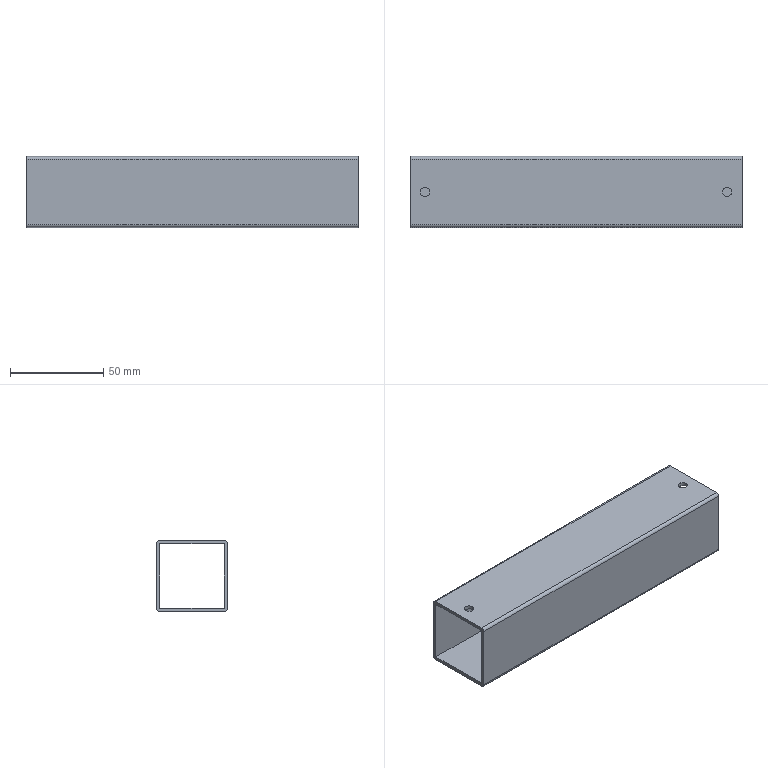Part | NX | features BREP 1 | 1 solid | 18 faces | box 177.8 x 38.1 x 38.1 mm | volume 47962 mm3 | plane 10 | cylinder 8 | commonest cylinder face diameters 3.175 x4 4.826 x2 5.029 x2
STEP:
#1=CARTESIAN_POINT('',(-88.9,19.05,-17.462));
#2=VERTEX_POINT('',#1);
#3=CARTESIAN_POINT('',(-88.9,19.05,17.462));
#4=VERTEX_POINT('',#3);
#5=CARTESIAN_POINT('',(-88.9,19.05,-17.462));
#6=DIRECTION('',(0.,0.,1.));
#7=VECTOR('',#6,1000.);
#8=LINE('',#5,#7);
#9=EDGE_CURVE('',#2,#4,#8,.T.);
#10=ORIENTED_EDGE('',*,*,#9,.F.);
#11=CARTESIAN_POINT('',(-88.9,17.462,-19.05));
#12=VERTEX_POINT('',#11);
#13=CARTESIAN_POINT('',(-88.9,17.462,-17.462));
#14=DIRECTION('',(-1.,0.,0.));
#15=DIRECTION('',(0.,1.,0.));
#16=AXIS2_PLACEMENT_3D('',#13,#14,#15);
#17=CIRCLE('',#16,1.587);
#18=EDGE_CURVE('',#2,#12,#17,.T.);
#19=ORIENTED_EDGE('',*,*,#18,.T.);
#20=CARTESIAN_POINT('',(-88.9,-17.462,-19.05));
#21=VERTEX_POINT('',#20);
#22=CARTESIAN_POINT('',(-88.9,-17.462,-19.05));
#23=DIRECTION('',(0.,1.,0.));
#24=VECTOR('',#23,1000.);
#25=LINE('',#22,#24);
#26=EDGE_CURVE('',#21,#12,#25,.T.);
#27=ORIENTED_EDGE('',*,*,#26,.F.);
#28=CARTESIAN_POINT('',(-88.9,-19.05,-17.462));
#29=VERTEX_POINT('',#28);
#30=CARTESIAN_POINT('',(-88.9,-17.462,-17.462));
#31=DIRECTION('',(-1.,0.,0.));
#32=DIRECTION('',(0.,0.,-1.));
#33=AXIS2_PLACEMENT_3D('',#30,#31,#32);
#34=CIRCLE('',#33,1.587);
#35=EDGE_CURVE('',#21,#29,#34,.T.);
#36=ORIENTED_EDGE('',*,*,#35,.T.);
#37=CARTESIAN_POINT('',(-88.9,-19.05,17.462));
#38=VERTEX_POINT('',#37);
#39=CARTESIAN_POINT('',(-88.9,-19.05,17.462));
#40=DIRECTION('',(0.,0.,-1.));
#41=VECTOR('',#40,1000.);
#42=LINE('',#39,#41);
#43=EDGE_CURVE('',#38,#29,#42,.T.);
#44=ORIENTED_EDGE('',*,*,#43,.F.);
#45=CARTESIAN_POINT('',(-88.9,-17.462,19.05));
#46=VERTEX_POINT('',#45);
#47=CARTESIAN_POINT('',(-88.9,-17.462,17.462));
#48=DIRECTION('',(-1.,0.,0.));
#49=DIRECTION('',(0.,-1.,0.));
#50=AXIS2_PLACEMENT_3D('',#47,#48,#49);
#51=CIRCLE('',#50,1.587);
#52=EDGE_CURVE('',#38,#46,#51,.T.);
#53=ORIENTED_EDGE('',*,*,#52,.T.);
#54=CARTESIAN_POINT('',(-88.9,17.462,19.05));
#55=VERTEX_POINT('',#54);
#56=CARTESIAN_POINT('',(-88.9,17.462,19.05));
#57=DIRECTION('',(0.,-1.,0.));
#58=VECTOR('',#57,1000.);
#59=LINE('',#56,#58);
#60=EDGE_CURVE('',#55,#46,#59,.T.);
#61=ORIENTED_EDGE('',*,*,#60,.F.);
#62=CARTESIAN_POINT('',(-88.9,17.462,17.462));
#63=DIRECTION('',(-1.,0.,0.));
#64=DIRECTION('',(0.,0.,1.));
#65=AXIS2_PLACEMENT_3D('',#62,#63,#64);
#66=CIRCLE('',#65,1.587);
#67=EDGE_CURVE('',#55,#4,#66,.T.);
#68=ORIENTED_EDGE('',*,*,#67,.T.);
#69=EDGE_LOOP('',(#10,#19,#27,#36,#44,#53,#61,#68));
#70=FACE_BOUND('',#69,.T.);
#71=CARTESIAN_POINT('',(-88.9,17.17,17.17));
#72=VERTEX_POINT('',#71);
#73=CARTESIAN_POINT('',(-88.9,17.17,-17.17));
#74=VERTEX_POINT('',#73);
#75=CARTESIAN_POINT('',(-88.9,17.17,17.17));
#76=DIRECTION('',(0.,0.,-1.));
#77=VECTOR('',#76,1000.);
#78=LINE('',#75,#77);
#79=EDGE_CURVE('',#72,#74,#78,.T.);
#80=ORIENTED_EDGE('',*,*,#79,.F.);
#81=CARTESIAN_POINT('',(-88.9,-17.17,17.17));
#82=VERTEX_POINT('',#81);
#83=CARTESIAN_POINT('',(-88.9,-17.17,17.17));
#84=DIRECTION('',(0.,1.,0.));
#85=VECTOR('',#84,1000.);
#86=LINE('',#83,#85);
#87=EDGE_CURVE('',#82,#72,#86,.T.);
#88=ORIENTED_EDGE('',*,*,#87,.F.);
#89=CARTESIAN_POINT('',(-88.9,-17.17,-17.17));
#90=VERTEX_POINT('',#89);
#91=CARTESIAN_POINT('',(-88.9,-17.17,-17.17));
#92=DIRECTION('',(0.,0.,1.));
#93=VECTOR('',#92,1000.);
#94=LINE('',#91,#93);
#95=EDGE_CURVE('',#90,#82,#94,.T.);
#96=ORIENTED_EDGE('',*,*,#95,.F.);
#97=CARTESIAN_POINT('',(-88.9,17.17,-17.17));
#98=DIRECTION('',(0.,-1.,0.));
#99=VECTOR('',#98,1000.);
#100=LINE('',#97,#99);
#101=EDGE_CURVE('',#74,#90,#100,.T.);
#102=ORIENTED_EDGE('',*,*,#101,.F.);
#103=EDGE_LOOP('',(#80,#88,#96,#102));
#104=FACE_BOUND('',#103,.T.);
#105=CARTESIAN_POINT('',(-88.9,0.,0.));
#106=DIRECTION('',(1.,0.,0.));
#107=DIRECTION('',(0.,1.,0.));
#108=AXIS2_PLACEMENT_3D('',#105,#106,#107);
#109=PLANE('',#108);
#110=ADVANCED_FACE('',(#70,#104),#109,.F.);
#111=CARTESIAN_POINT('',(88.9,-17.17,-17.17));
#112=VERTEX_POINT('',#111);
#113=CARTESIAN_POINT('',(-88.9,-17.17,-17.17));
#114=DIRECTION('',(1.,0.,0.));
#115=VECTOR('',#114,1000.);
#116=LINE('',#113,#115);
#117=EDGE_CURVE('',#90,#112,#116,.T.);
#118=ORIENTED_EDGE('',*,*,#117,.T.);
#119=CARTESIAN_POINT('',(88.9,17.17,-17.17));
#120=VERTEX_POINT('',#119);
#121=CARTESIAN_POINT('',(88.9,17.17,-17.17));
#122=DIRECTION('',(0.,-1.,0.));
#123=VECTOR('',#122,1000.);
#124=LINE('',#121,#123);
#125=EDGE_CURVE('',#120,#112,#124,.T.);
#126=ORIENTED_EDGE('',*,*,#125,.F.);
#127=CARTESIAN_POINT('',(-88.9,17.17,-17.17));
#128=DIRECTION('',(1.,0.,0.));
#129=VECTOR('',#128,1000.);
#130=LINE('',#127,#129);
#131=EDGE_CURVE('',#74,#120,#130,.T.);
#132=ORIENTED_EDGE('',*,*,#131,.F.);
#133=ORIENTED_EDGE('',*,*,#101,.T.);
#134=EDGE_LOOP('',(#118,#126,#132,#133));
#135=FACE_BOUND('',#134,.T.);
#136=CARTESIAN_POINT('',(-88.9,17.17,-17.17));
#137=DIRECTION('',(0.,0.,1.));
#138=DIRECTION('',(1.,0.,0.));
#139=AXIS2_PLACEMENT_3D('',#136,#137,#138);
#140=PLANE('',#139);
#141=ADVANCED_FACE('',(#135),#140,.T.);
#142=ORIENTED_EDGE('',*,*,#131,.T.);
#143=CARTESIAN_POINT('',(88.9,17.17,17.17));
#144=VERTEX_POINT('',#143);
#145=CARTESIAN_POINT('',(88.9,17.17,17.17));
#146=DIRECTION('',(0.,0.,-1.));
#147=VECTOR('',#146,1000.);
#148=LINE('',#145,#147);
#149=EDGE_CURVE('',#144,#120,#148,.T.);
#150=ORIENTED_EDGE('',*,*,#149,.F.);
#151=CARTESIAN_POINT('',(-88.9,17.17,17.17));
#152=DIRECTION('',(1.,0.,0.));
#153=VECTOR('',#152,1000.);
#154=LINE('',#151,#153);
#155=EDGE_CURVE('',#72,#144,#154,.T.);
#156=ORIENTED_EDGE('',*,*,#155,.F.);
#157=ORIENTED_EDGE('',*,*,#79,.T.);
#158=EDGE_LOOP('',(#142,#150,#156,#157));
#159=FACE_BOUND('',#158,.T.);
#160=CARTESIAN_POINT('',(-88.9,17.17,17.17));
#161=DIRECTION('',(0.,-1.,0.));
#162=DIRECTION('',(0.,0.,-1.));
#163=AXIS2_PLACEMENT_3D('',#160,#161,#162);
#164=PLANE('',#163);
#165=ADVANCED_FACE('',(#159),#164,.T.);
#166=ORIENTED_EDGE('',*,*,#155,.T.);
#167=CARTESIAN_POINT('',(88.9,-17.17,17.17));
#168=VERTEX_POINT('',#167);
#169=CARTESIAN_POINT('',(88.9,-17.17,17.17));
#170=DIRECTION('',(0.,1.,0.));
#171=VECTOR('',#170,1000.);
#172=LINE('',#169,#171);
#173=EDGE_CURVE('',#168,#144,#172,.T.);
#174=ORIENTED_EDGE('',*,*,#173,.F.);
#175=CARTESIAN_POINT('',(-88.9,-17.17,17.17));
#176=DIRECTION('',(1.,0.,0.));
#177=VECTOR('',#176,1000.);
#178=LINE('',#175,#177);
#179=EDGE_CURVE('',#82,#168,#178,.T.);
#180=ORIENTED_EDGE('',*,*,#179,.F.);
#181=ORIENTED_EDGE('',*,*,#87,.T.);
#182=EDGE_LOOP('',(#166,#174,#180,#181));
#183=FACE_BOUND('',#182,.T.);
#184=CARTESIAN_POINT('',(83.312,0.,17.17));
#185=VERTEX_POINT('',#184);
#186=CARTESIAN_POINT('',(78.486,0.,17.17));
#187=VERTEX_POINT('',#186);
#188=CARTESIAN_POINT('',(80.899,0.,17.17));
#189=DIRECTION('',(0.,0.,-1.));
#190=DIRECTION('',(1.,0.,0.));
#191=AXIS2_PLACEMENT_3D('',#188,#189,#190);
#192=CIRCLE('',#191,2.413);
#193=EDGE_CURVE('',#185,#187,#192,.T.);
#194=ORIENTED_EDGE('',*,*,#193,.F.);
#195=CARTESIAN_POINT('',(80.899,0.,17.17));
#196=DIRECTION('',(0.,0.,-1.));
#197=DIRECTION('',(-1.,0.,0.));
#198=AXIS2_PLACEMENT_3D('',#195,#196,#197);
#199=CIRCLE('',#198,2.413);
#200=EDGE_CURVE('',#187,#185,#199,.T.);
#201=ORIENTED_EDGE('',*,*,#200,.F.);
#202=EDGE_LOOP('',(#194,#201));
#203=FACE_BOUND('',#202,.T.);
#204=CARTESIAN_POINT('',(-78.384,0.,17.17));
#205=VERTEX_POINT('',#204);
#206=CARTESIAN_POINT('',(-83.414,0.,17.17));
#207=VERTEX_POINT('',#206);
#208=CARTESIAN_POINT('',(-80.899,0.,17.17));
#209=DIRECTION('',(0.,0.,-1.));
#210=DIRECTION('',(1.,0.,0.));
#211=AXIS2_PLACEMENT_3D('',#208,#209,#210);
#212=CIRCLE('',#211,2.515);
#213=EDGE_CURVE('',#205,#207,#212,.T.);
#214=ORIENTED_EDGE('',*,*,#213,.F.);
#215=CARTESIAN_POINT('',(-80.899,0.,17.17));
#216=DIRECTION('',(0.,0.,-1.));
#217=DIRECTION('',(-1.,0.,0.));
#218=AXIS2_PLACEMENT_3D('',#215,#216,#217);
#219=CIRCLE('',#218,2.515);
#220=EDGE_CURVE('',#207,#205,#219,.T.);
#221=ORIENTED_EDGE('',*,*,#220,.F.);
#222=EDGE_LOOP('',(#214,#221));
#223=FACE_BOUND('',#222,.T.);
#224=CARTESIAN_POINT('',(-88.9,-17.17,17.17));
#225=DIRECTION('',(0.,0.,-1.));
#226=DIRECTION('',(0.,-1.,0.));
#227=AXIS2_PLACEMENT_3D('',#224,#225,#226);
#228=PLANE('',#227);
#229=ADVANCED_FACE('',(#183,#203,#223),#228,.T.);
#230=ORIENTED_EDGE('',*,*,#179,.T.);
#231=CARTESIAN_POINT('',(88.9,-17.17,-17.17));
#232=DIRECTION('',(0.,0.,1.));
#233=VECTOR('',#232,1000.);
#234=LINE('',#231,#233);
#235=EDGE_CURVE('',#112,#168,#234,.T.);
#236=ORIENTED_EDGE('',*,*,#235,.F.);
#237=ORIENTED_EDGE('',*,*,#117,.F.);
#238=ORIENTED_EDGE('',*,*,#95,.T.);
#239=EDGE_LOOP('',(#230,#236,#237,#238));
#240=FACE_BOUND('',#239,.T.);
#241=CARTESIAN_POINT('',(-88.9,-17.17,-17.17));
#242=DIRECTION('',(0.,1.,0.));
#243=DIRECTION('',(1.,0.,0.));
#244=AXIS2_PLACEMENT_3D('',#241,#242,#243);
#245=PLANE('',#244);
#246=ADVANCED_FACE('',(#240),#245,.T.);
#247=CARTESIAN_POINT('',(88.9,17.462,19.05));
#248=VERTEX_POINT('',#247);
#249=CARTESIAN_POINT('',(88.9,-17.462,19.05));
#250=VERTEX_POINT('',#249);
#251=CARTESIAN_POINT('',(88.9,17.462,19.05));
#252=DIRECTION('',(0.,-1.,0.));
#253=VECTOR('',#252,1000.);
#254=LINE('',#251,#253);
#255=EDGE_CURVE('',#248,#250,#254,.T.);
#256=ORIENTED_EDGE('',*,*,#255,.T.);
#257=CARTESIAN_POINT('',(88.9,-19.05,17.462));
#258=VERTEX_POINT('',#257);
#259=CARTESIAN_POINT('',(88.9,-17.462,17.462));
#260=DIRECTION('',(1.,0.,0.));
#261=DIRECTION('',(0.,0.,1.));
#262=AXIS2_PLACEMENT_3D('',#259,#260,#261);
#263=CIRCLE('',#262,1.587);
#264=EDGE_CURVE('',#250,#258,#263,.T.);
#265=ORIENTED_EDGE('',*,*,#264,.T.);
#266=CARTESIAN_POINT('',(88.9,-19.05,-17.462));
#267=VERTEX_POINT('',#266);
#268=CARTESIAN_POINT('',(88.9,-19.05,17.462));
#269=DIRECTION('',(0.,0.,-1.));
#270=VECTOR('',#269,1000.);
#271=LINE('',#268,#270);
#272=EDGE_CURVE('',#258,#267,#271,.T.);
#273=ORIENTED_EDGE('',*,*,#272,.T.);
#274=CARTESIAN_POINT('',(88.9,-17.462,-19.05));
#275=VERTEX_POINT('',#274);
#276=CARTESIAN_POINT('',(88.9,-17.462,-17.462));
#277=DIRECTION('',(1.,0.,0.));
#278=DIRECTION('',(0.,-1.,0.));
#279=AXIS2_PLACEMENT_3D('',#276,#277,#278);
#280=CIRCLE('',#279,1.587);
#281=EDGE_CURVE('',#267,#275,#280,.T.);
#282=ORIENTED_EDGE('',*,*,#281,.T.);
#283=CARTESIAN_POINT('',(88.9,17.462,-19.05));
#284=VERTEX_POINT('',#283);
#285=CARTESIAN_POINT('',(88.9,-17.462,-19.05));
#286=DIRECTION('',(0.,1.,0.));
#287=VECTOR('',#286,1000.);
#288=LINE('',#285,#287);
#289=EDGE_CURVE('',#275,#284,#288,.T.);
#290=ORIENTED_EDGE('',*,*,#289,.T.);
#291=CARTESIAN_POINT('',(88.9,19.05,-17.462));
#292=VERTEX_POINT('',#291);
#293=CARTESIAN_POINT('',(88.9,17.462,-17.462));
#294=DIRECTION('',(1.,0.,0.));
#295=DIRECTION('',(0.,0.,-1.));
#296=AXIS2_PLACEMENT_3D('',#293,#294,#295);
#297=CIRCLE('',#296,1.587);
#298=EDGE_CURVE('',#284,#292,#297,.T.);
#299=ORIENTED_EDGE('',*,*,#298,.T.);
#300=CARTESIAN_POINT('',(88.9,19.05,17.462));
#301=VERTEX_POINT('',#300);
#302=CARTESIAN_POINT('',(88.9,19.05,-17.462));
#303=DIRECTION('',(0.,0.,1.));
#304=VECTOR('',#303,1000.);
#305=LINE('',#302,#304);
#306=EDGE_CURVE('',#292,#301,#305,.T.);
#307=ORIENTED_EDGE('',*,*,#306,.T.);
#308=CARTESIAN_POINT('',(88.9,17.462,17.462));
#309=DIRECTION('',(1.,0.,0.));
#310=DIRECTION('',(0.,1.,0.));
#311=AXIS2_PLACEMENT_3D('',#308,#309,#310);
#312=CIRCLE('',#311,1.587);
#313=EDGE_CURVE('',#301,#248,#312,.T.);
#314=ORIENTED_EDGE('',*,*,#313,.T.);
#315=EDGE_LOOP('',(#256,#265,#273,#282,#290,#299,#307,#314));
#316=FACE_BOUND('',#315,.T.);
#317=ORIENTED_EDGE('',*,*,#235,.T.);
#318=ORIENTED_EDGE('',*,*,#173,.T.);
#319=ORIENTED_EDGE('',*,*,#149,.T.);
#320=ORIENTED_EDGE('',*,*,#125,.T.);
#321=EDGE_LOOP('',(#317,#318,#319,#320));
#322=FACE_BOUND('',#321,.T.);
#323=CARTESIAN_POINT('',(88.9,0.,0.));
#324=DIRECTION('',(1.,0.,0.));
#325=DIRECTION('',(0.,1.,0.));
#326=AXIS2_PLACEMENT_3D('',#323,#324,#325);
#327=PLANE('',#326);
#328=ADVANCED_FACE('',(#316,#322),#327,.T.);
#329=ORIENTED_EDGE('',*,*,#313,.F.);
#330=CARTESIAN_POINT('',(88.9,19.05,17.462));
#331=DIRECTION('',(-1.,0.,0.));
#332=VECTOR('',#331,1000.);
#333=LINE('',#330,#332);
#334=EDGE_CURVE('',#301,#4,#333,.T.);
#335=ORIENTED_EDGE('',*,*,#334,.T.);
#336=ORIENTED_EDGE('',*,*,#67,.F.);
#337=CARTESIAN_POINT('',(88.9,17.462,19.05));
#338=DIRECTION('',(-1.,0.,0.));
#339=VECTOR('',#338,1000.);
#340=LINE('',#337,#339);
#341=EDGE_CURVE('',#248,#55,#340,.T.);
#342=ORIENTED_EDGE('',*,*,#341,.F.);
#343=EDGE_LOOP('',(#329,#335,#336,#342));
#344=FACE_BOUND('',#343,.T.);
#345=CARTESIAN_POINT('',(89.191,17.462,17.462));
#346=DIRECTION('',(-1.,0.,0.));
#347=DIRECTION('',(0.,0.,1.));
#348=AXIS2_PLACEMENT_3D('',#345,#346,#347);
#349=CYLINDRICAL_SURFACE('',#348,1.587);
#350=ADVANCED_FACE('',(#344),#349,.T.);
#351=ORIENTED_EDGE('',*,*,#60,.T.);
#352=CARTESIAN_POINT('',(88.9,-17.462,19.05));
#353=DIRECTION('',(-1.,0.,0.));
#354=VECTOR('',#353,1000.);
#355=LINE('',#352,#354);
#356=EDGE_CURVE('',#250,#46,#355,.T.);
#357=ORIENTED_EDGE('',*,*,#356,.F.);
#358=ORIENTED_EDGE('',*,*,#255,.F.);
#359=ORIENTED_EDGE('',*,*,#341,.T.);
#360=EDGE_LOOP('',(#351,#357,#358,#359));
#361=FACE_BOUND('',#360,.T.);
#362=CARTESIAN_POINT('',(83.312,0.,19.05));
#363=VERTEX_POINT('',#362);
#364=CARTESIAN_POINT('',(78.486,0.,19.05));
#365=VERTEX_POINT('',#364);
#366=CARTESIAN_POINT('',(80.899,0.,19.05));
#367=DIRECTION('',(0.,0.,-1.));
#368=DIRECTION('',(1.,0.,0.));
#369=AXIS2_PLACEMENT_3D('',#366,#367,#368);
#370=CIRCLE('',#369,2.413);
#371=EDGE_CURVE('',#363,#365,#370,.T.);
#372=ORIENTED_EDGE('',*,*,#371,.T.);
#373=CARTESIAN_POINT('',(80.899,0.,19.05));
#374=DIRECTION('',(0.,0.,-1.));
#375=DIRECTION('',(-1.,0.,0.));
#376=AXIS2_PLACEMENT_3D('',#373,#374,#375);
#377=CIRCLE('',#376,2.413);
#378=EDGE_CURVE('',#365,#363,#377,.T.);
#379=ORIENTED_EDGE('',*,*,#378,.T.);
#380=EDGE_LOOP('',(#372,#379));
#381=FACE_BOUND('',#380,.T.);
#382=CARTESIAN_POINT('',(-78.384,0.,19.05));
#383=VERTEX_POINT('',#382);
#384=CARTESIAN_POINT('',(-83.414,0.,19.05));
#385=VERTEX_POINT('',#384);
#386=CARTESIAN_POINT('',(-80.899,0.,19.05));
#387=DIRECTION('',(0.,0.,-1.));
#388=DIRECTION('',(1.,0.,0.));
#389=AXIS2_PLACEMENT_3D('',#386,#387,#388);
#390=CIRCLE('',#389,2.515);
#391=EDGE_CURVE('',#383,#385,#390,.T.);
#392=ORIENTED_EDGE('',*,*,#391,.T.);
#393=CARTESIAN_POINT('',(-80.899,0.,19.05));
#394=DIRECTION('',(0.,0.,-1.));
#395=DIRECTION('',(-1.,0.,0.));
#396=AXIS2_PLACEMENT_3D('',#393,#394,#395);
#397=CIRCLE('',#396,2.515);
#398=EDGE_CURVE('',#385,#383,#397,.T.);
#399=ORIENTED_EDGE('',*,*,#398,.T.);
#400=EDGE_LOOP('',(#392,#399));
#401=FACE_BOUND('',#400,.T.);
#402=CARTESIAN_POINT('',(-88.9,19.05,19.05));
#403=DIRECTION('',(0.,0.,1.));
#404=DIRECTION('',(1.,0.,0.));
#405=AXIS2_PLACEMENT_3D('',#402,#403,#404);
#406=PLANE('',#405);
#407=ADVANCED_FACE('',(#361,#381,#401),#406,.T.);
#408=ORIENTED_EDGE('',*,*,#264,.F.);
#409=ORIENTED_EDGE('',*,*,#356,.T.);
#410=ORIENTED_EDGE('',*,*,#52,.F.);
#411=CARTESIAN_POINT('',(88.9,-19.05,17.462));
#412=DIRECTION('',(-1.,0.,0.));
#413=VECTOR('',#412,1000.);
#414=LINE('',#411,#413);
#415=EDGE_CURVE('',#258,#38,#414,.T.);
#416=ORIENTED_EDGE('',*,*,#415,.F.);
#417=EDGE_LOOP('',(#408,#409,#410,#416));
#418=FACE_BOUND('',#417,.T.);
#419=CARTESIAN_POINT('',(89.191,-17.462,17.462));
#420=DIRECTION('',(-1.,0.,0.));
#421=DIRECTION('',(0.,-1.,0.));
#422=AXIS2_PLACEMENT_3D('',#419,#420,#421);
#423=CYLINDRICAL_SURFACE('',#422,1.587);
#424=ADVANCED_FACE('',(#418),#423,.T.);
#425=ORIENTED_EDGE('',*,*,#43,.T.);
#426=CARTESIAN_POINT('',(88.9,-19.05,-17.462));
#427=DIRECTION('',(-1.,0.,0.));
#428=VECTOR('',#427,1000.);
#429=LINE('',#426,#428);
#430=EDGE_CURVE('',#267,#29,#429,.T.);
#431=ORIENTED_EDGE('',*,*,#430,.F.);
#432=ORIENTED_EDGE('',*,*,#272,.F.);
#433=ORIENTED_EDGE('',*,*,#415,.T.);
#434=EDGE_LOOP('',(#425,#431,#432,#433));
#435=FACE_BOUND('',#434,.T.);
#436=CARTESIAN_POINT('',(-88.9,-19.05,19.05));
#437=DIRECTION('',(0.,-1.,0.));
#438=DIRECTION('',(0.,0.,-1.));
#439=AXIS2_PLACEMENT_3D('',#436,#437,#438);
#440=PLANE('',#439);
#441=ADVANCED_FACE('',(#435),#440,.T.);
#442=ORIENTED_EDGE('',*,*,#281,.F.);
#443=ORIENTED_EDGE('',*,*,#430,.T.);
#444=ORIENTED_EDGE('',*,*,#35,.F.);
#445=CARTESIAN_POINT('',(88.9,-17.462,-19.05));
#446=DIRECTION('',(-1.,0.,0.));
#447=VECTOR('',#446,1000.);
#448=LINE('',#445,#447);
#449=EDGE_CURVE('',#275,#21,#448,.T.);
#450=ORIENTED_EDGE('',*,*,#449,.F.);
#451=EDGE_LOOP('',(#442,#443,#444,#450));
#452=FACE_BOUND('',#451,.T.);
#453=CARTESIAN_POINT('',(89.191,-17.462,-17.462));
#454=DIRECTION('',(-1.,0.,0.));
#455=DIRECTION('',(0.,0.,-1.));
#456=AXIS2_PLACEMENT_3D('',#453,#454,#455);
#457=CYLINDRICAL_SURFACE('',#456,1.587);
#458=ADVANCED_FACE('',(#452),#457,.T.);
#459=ORIENTED_EDGE('',*,*,#289,.F.);
#460=ORIENTED_EDGE('',*,*,#449,.T.);
#461=ORIENTED_EDGE('',*,*,#26,.T.);
#462=CARTESIAN_POINT('',(88.9,17.462,-19.05));
#463=DIRECTION('',(-1.,0.,0.));
#464=VECTOR('',#463,1000.);
#465=LINE('',#462,#464);
#466=EDGE_CURVE('',#284,#12,#465,.T.);
#467=ORIENTED_EDGE('',*,*,#466,.F.);
#468=EDGE_LOOP('',(#459,#460,#461,#467));
#469=FACE_BOUND('',#468,.T.);
#470=CARTESIAN_POINT('',(-88.9,-19.05,-19.05));
#471=DIRECTION('',(0.,0.,-1.));
#472=DIRECTION('',(0.,-1.,0.));
#473=AXIS2_PLACEMENT_3D('',#470,#471,#472);
#474=PLANE('',#473);
#475=ADVANCED_FACE('',(#469),#474,.T.);
#476=ORIENTED_EDGE('',*,*,#298,.F.);
#477=ORIENTED_EDGE('',*,*,#466,.T.);
#478=ORIENTED_EDGE('',*,*,#18,.F.);
#479=CARTESIAN_POINT('',(88.9,19.05,-17.462));
#480=DIRECTION('',(-1.,0.,0.));
#481=VECTOR('',#480,1000.);
#482=LINE('',#479,#481);
#483=EDGE_CURVE('',#292,#2,#482,.T.);
#484=ORIENTED_EDGE('',*,*,#483,.F.);
#485=EDGE_LOOP('',(#476,#477,#478,#484));
#486=FACE_BOUND('',#485,.T.);
#487=CARTESIAN_POINT('',(89.191,17.462,-17.462));
#488=DIRECTION('',(-1.,0.,0.));
#489=DIRECTION('',(0.,1.,0.));
#490=AXIS2_PLACEMENT_3D('',#487,#488,#489);
#491=CYLINDRICAL_SURFACE('',#490,1.587);
#492=ADVANCED_FACE('',(#486),#491,.T.);
#493=ORIENTED_EDGE('',*,*,#306,.F.);
#494=ORIENTED_EDGE('',*,*,#483,.T.);
#495=ORIENTED_EDGE('',*,*,#9,.T.);
#496=ORIENTED_EDGE('',*,*,#334,.F.);
#497=EDGE_LOOP('',(#493,#494,#495,#496));
#498=FACE_BOUND('',#497,.T.);
#499=CARTESIAN_POINT('',(-88.9,19.05,-19.05));
#500=DIRECTION('',(0.,1.,0.));
#501=DIRECTION('',(1.,0.,0.));
#502=AXIS2_PLACEMENT_3D('',#499,#500,#501);
#503=PLANE('',#502);
#504=ADVANCED_FACE('',(#498),#503,.T.);
#505=CARTESIAN_POINT('',(78.486,0.,19.05));
#506=DIRECTION('',(0.,0.,-1.));
#507=VECTOR('',#506,1000.);
#508=LINE('',#505,#507);
#509=EDGE_CURVE('',#365,#187,#508,.T.);
#510=ORIENTED_EDGE('',*,*,#509,.T.);
#511=ORIENTED_EDGE('',*,*,#200,.T.);
#512=CARTESIAN_POINT('',(83.312,0.,19.05));
#513=DIRECTION('',(0.,0.,-1.));
#514=VECTOR('',#513,1000.);
#515=LINE('',#512,#514);
#516=EDGE_CURVE('',#363,#185,#515,.T.);
#517=ORIENTED_EDGE('',*,*,#516,.F.);
#518=ORIENTED_EDGE('',*,*,#378,.F.);
#519=EDGE_LOOP('',(#510,#511,#517,#518));
#520=FACE_BOUND('',#519,.T.);
#521=CARTESIAN_POINT('',(80.899,0.,19.05));
#522=DIRECTION('',(0.,0.,-1.));
#523=DIRECTION('',(-1.,0.,0.));
#524=AXIS2_PLACEMENT_3D('',#521,#522,#523);
#525=CYLINDRICAL_SURFACE('',#524,2.413);
#526=ADVANCED_FACE('',(#520),#525,.F.);
#527=ORIENTED_EDGE('',*,*,#516,.T.);
#528=ORIENTED_EDGE('',*,*,#193,.T.);
#529=ORIENTED_EDGE('',*,*,#509,.F.);
#530=ORIENTED_EDGE('',*,*,#371,.F.);
#531=EDGE_LOOP('',(#527,#528,#529,#530));
#532=FACE_BOUND('',#531,.T.);
#533=CARTESIAN_POINT('',(80.899,0.,19.05));
#534=DIRECTION('',(0.,0.,-1.));
#535=DIRECTION('',(-1.,0.,0.));
#536=AXIS2_PLACEMENT_3D('',#533,#534,#535);
#537=CYLINDRICAL_SURFACE('',#536,2.413);
#538=ADVANCED_FACE('',(#532),#537,.F.);
#539=CARTESIAN_POINT('',(-83.414,0.,19.05));
#540=DIRECTION('',(0.,0.,-1.));
#541=VECTOR('',#540,1000.);
#542=LINE('',#539,#541);
#543=EDGE_CURVE('',#385,#207,#542,.T.);
#544=ORIENTED_EDGE('',*,*,#543,.T.);
#545=ORIENTED_EDGE('',*,*,#220,.T.);
#546=CARTESIAN_POINT('',(-78.384,0.,19.05));
#547=DIRECTION('',(0.,0.,-1.));
#548=VECTOR('',#547,1000.);
#549=LINE('',#546,#548);
#550=EDGE_CURVE('',#383,#205,#549,.T.);
#551=ORIENTED_EDGE('',*,*,#550,.F.);
#552=ORIENTED_EDGE('',*,*,#398,.F.);
#553=EDGE_LOOP('',(#544,#545,#551,#552));
#554=FACE_BOUND('',#553,.T.);
#555=CARTESIAN_POINT('',(-80.899,0.,19.05));
#556=DIRECTION('',(0.,0.,-1.));
#557=DIRECTION('',(-1.,0.,0.));
#558=AXIS2_PLACEMENT_3D('',#555,#556,#557);
#559=CYLINDRICAL_SURFACE('',#558,2.515);
#560=ADVANCED_FACE('',(#554),#559,.F.);
#561=ORIENTED_EDGE('',*,*,#550,.T.);
#562=ORIENTED_EDGE('',*,*,#213,.T.);
#563=ORIENTED_EDGE('',*,*,#543,.F.);
#564=ORIENTED_EDGE('',*,*,#391,.F.);
#565=EDGE_LOOP('',(#561,#562,#563,#564));
#566=FACE_BOUND('',#565,.T.);
#567=CARTESIAN_POINT('',(-80.899,0.,19.05));
#568=DIRECTION('',(0.,0.,-1.));
#569=DIRECTION('',(-1.,0.,0.));
#570=AXIS2_PLACEMENT_3D('',#567,#568,#569);
#571=CYLINDRICAL_SURFACE('',#570,2.515);
#572=ADVANCED_FACE('',(#566),#571,.F.);
#573=CLOSED_SHELL('',(#110,#141,#165,#229,#246,#328,#350,#407,#424,#441,#458,#475,#492,#504,#526,#538,#560,#572));
#574=MANIFOLD_SOLID_BREP('',#573);
#575=(LENGTH_UNIT()NAMED_UNIT(*)SI_UNIT(.MILLI.,.METRE.));
#576=UNCERTAINTY_MEASURE_WITH_UNIT(LENGTH_MEASURE(0.00001),#575,'','');
#577=(NAMED_UNIT(*)PLANE_ANGLE_UNIT()SI_UNIT($,.RADIAN.));
#578=(NAMED_UNIT(*)SI_UNIT($,.STERADIAN.)SOLID_ANGLE_UNIT());
#579=(GEOMETRIC_REPRESENTATION_CONTEXT(3)GLOBAL_UNCERTAINTY_ASSIGNED_CONTEXT((#576))GLOBAL_UNIT_ASSIGNED_CONTEXT((#575,#577,#578))REPRESENTATION_CONTEXT('',''));
#580=ADVANCED_BREP_SHAPE_REPRESENTATION('',(#574),#579);